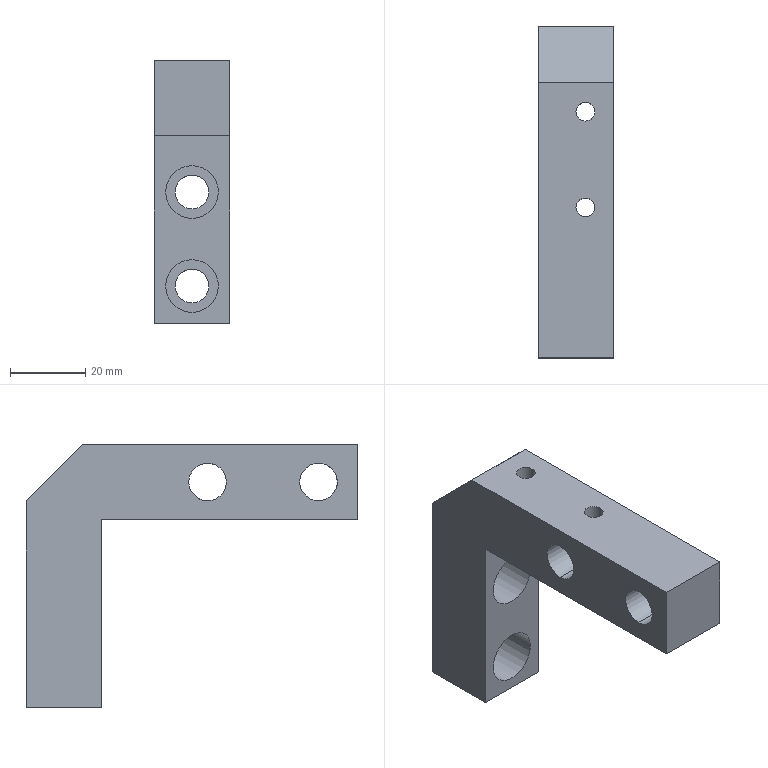Part | STEP file | Positioning_id2254_x_t | 1 solid | 34 faces | box 20 x 88.297 x 69.995 mm | volume 43755 mm3 | cylinder 22 | plane 12 | commonest cylinder face diameters 5 x8 10 x6 9 x4 14 x4